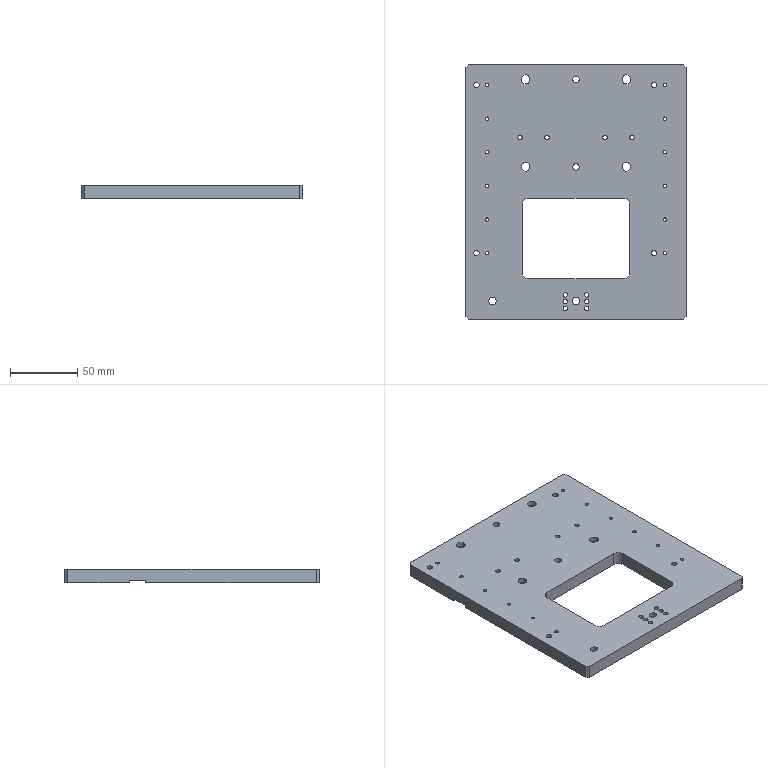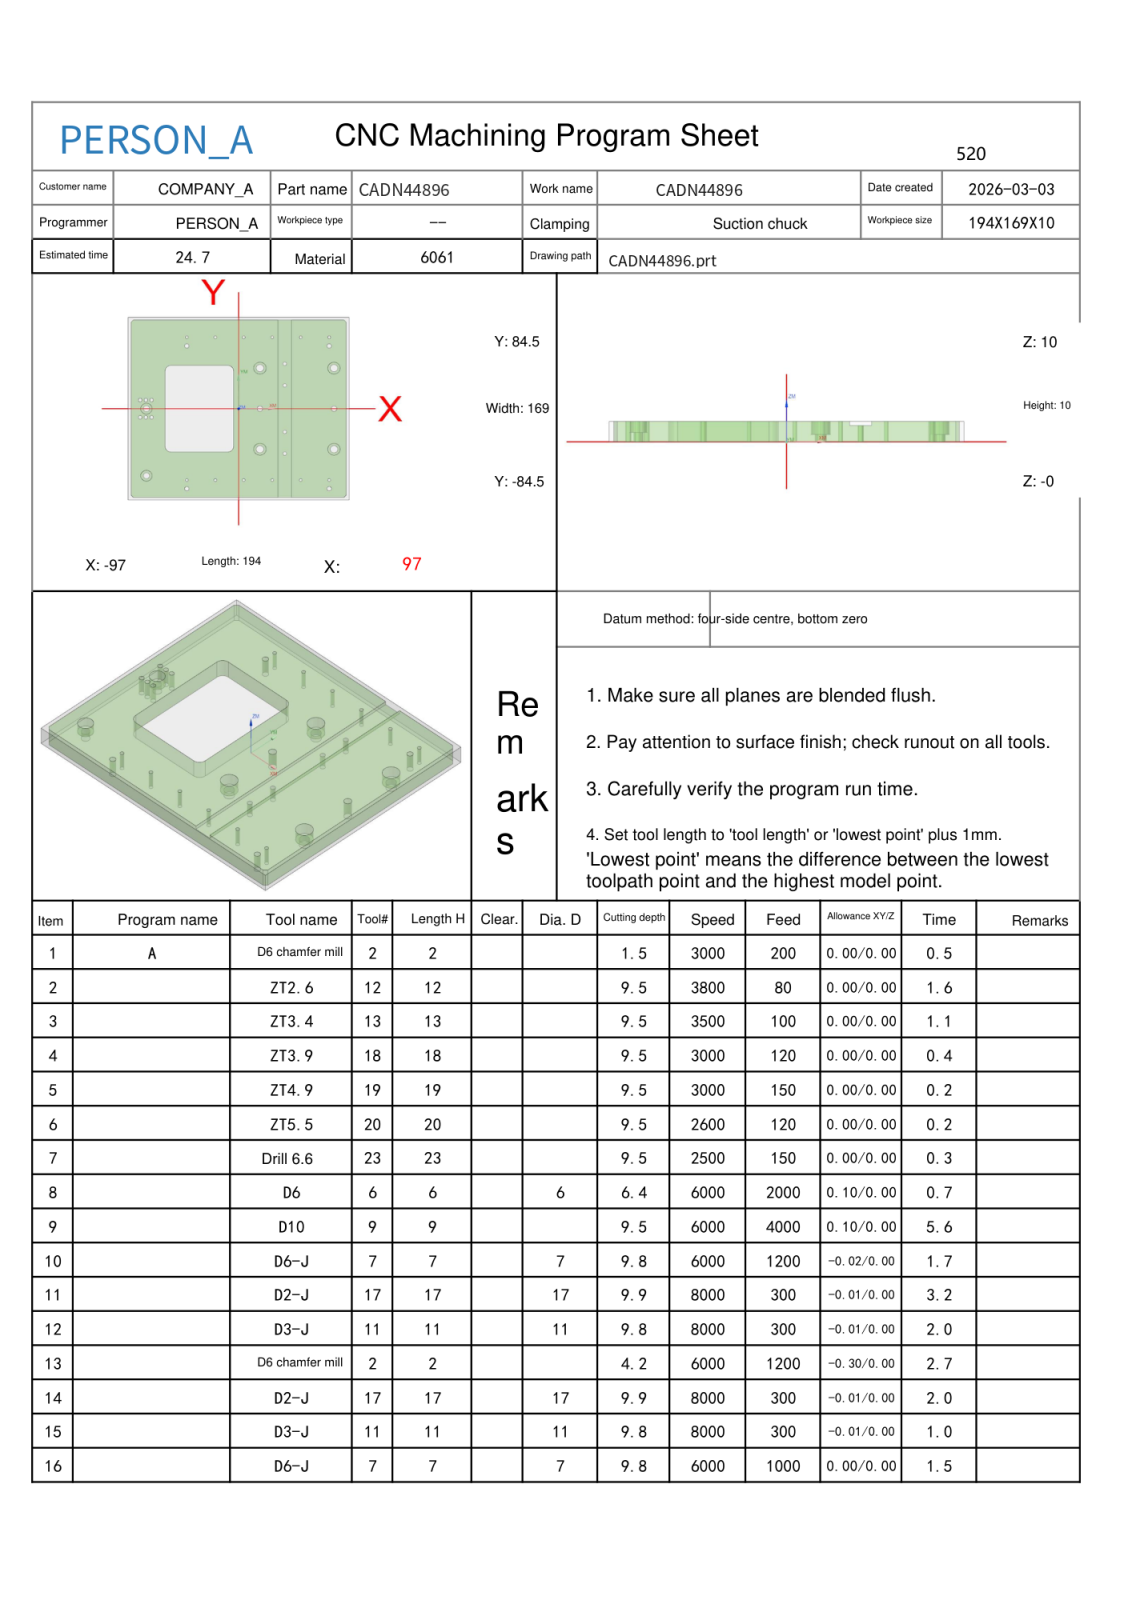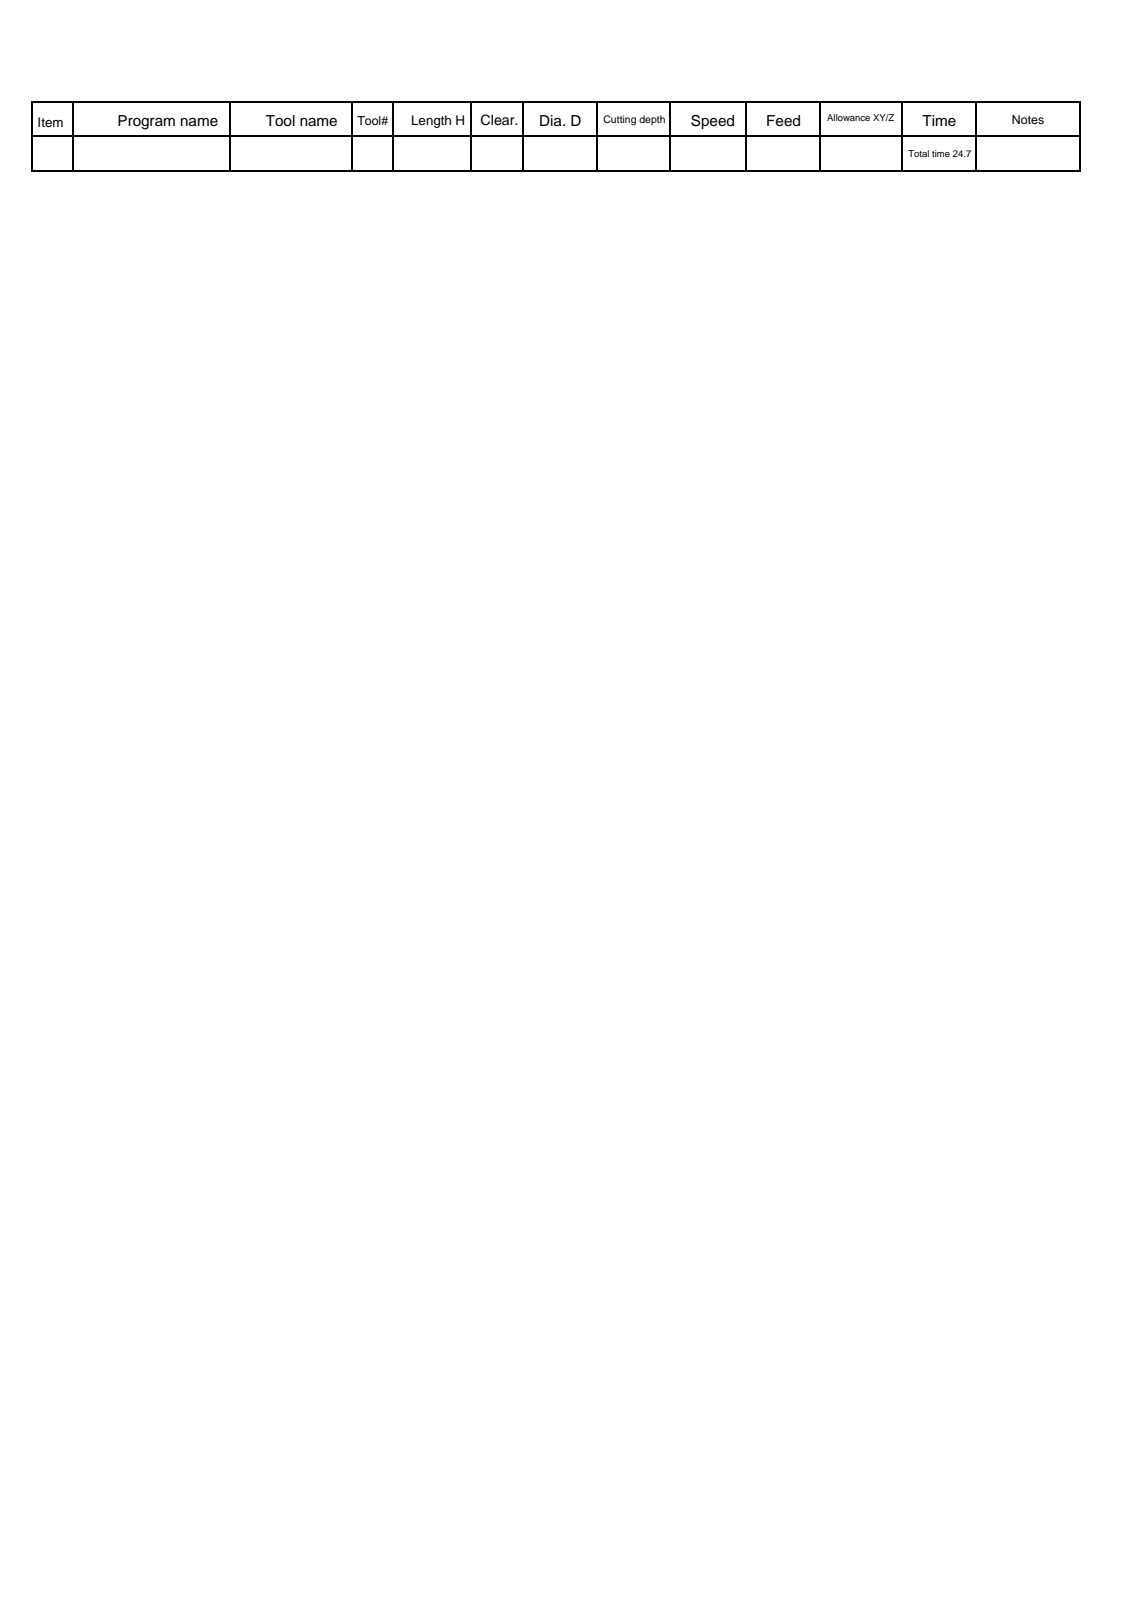NC program | NX | posted by the shop | part box 164 x 189 x 10 mm
Lines 1039 to 2443 of 4061, first 1137 of 1405 lines:
N11 T17 M06
(D2-J  D=2. R=0. H=17 ce=-0.01 di=0.00)
(D.N=17 MAX_Z=40. MIN_Z=0.15 Time=3.12M)
G00 G90 G54 X-75.935 Y8.28 M03 S8000
G43 H17 Z40.
M08
Z10.5
G01 X-76.054 Y8.446 Z10.489 F300.
X-76.222 Y8.566 Z10.478
X-76.421 Y8.626 Z10.468
X-76.579 Z10.459
X-76.77 Y8.57 Z10.449
X-76.933 Y8.458 Z10.439
X-77.054 Y8.301 Z10.428
X-77.12 Y8.114 Z10.418
X-77.126 Y7.921 Z10.408
X-77.066 Y7.722 Z10.397
X-76.946 Y7.554 Z10.386
X-76.778 Y7.434 Z10.375
X-76.579 Y7.374 Z10.364
X-76.421 Z10.356
X-76.222 Y7.434 Z10.345
X-76.054 Y7.554 Z10.334
X-75.934 Y7.722 Z10.323
X-75.874 Y7.921 Z10.313
Y8.079 Z10.304
X-75.934 Y8.278 Z10.293
X-76.054 Y8.446 Z10.282
X-76.222 Y8.566 Z10.272
X-76.421 Y8.626 Z10.261
X-76.579 Z10.252
X-76.77 Y8.57 Z10.242
X-76.933 Y8.458 Z10.232
X-77.054 Y8.301 Z10.221
X-77.12 Y8.114 Z10.211
X-77.126 Y7.921 Z10.201
X-77.066 Y7.722 Z10.19
X-76.946 Y7.554 Z10.179
X-76.778 Y7.434 Z10.168
X-76.579 Y7.374 Z10.157
X-76.421 Z10.149
X-76.222 Y7.434 Z10.138
X-76.054 Y7.554 Z10.127
X-75.934 Y7.722 Z10.117
X-75.874 Y7.921 Z10.106
Y8.079 Z10.097
X-75.934 Y8.278 Z10.087
X-76.054 Y8.446 Z10.076
X-76.222 Y8.566 Z10.065
X-76.421 Y8.626 Z10.054
X-76.579 Z10.046
X-76.77 Y8.57 Z10.035
X-76.933 Y8.458 Z10.025
X-77.054 Y8.301 Z10.015
X-77.12 Y8.114 Z10.004
X-77.125 Y8.035 Z10.
G41 D17
X-77.16 Y8.
G03 X-76.5 Y7.34 Z9.877 I.66 J0.0
X-75.84 Y8. Z9.754 I0.0 J.66
X-76.5 Y8.66 Z9.631 I-.66 J0.0
X-77.16 Y8. Z9.508 I0.0 J-.66
X-76.5 Y7.34 Z9.384 I.66 J0.0
X-75.84 Y8. Z9.261 I0.0 J.66
X-76.5 Y8.66 Z9.138 I-.66 J0.0
X-77.16 Y8. Z9.015 I0.0 J-.66
X-76.5 Y7.34 Z8.892 I.66 J0.0
X-75.84 Y8. Z8.769 I0.0 J.66
X-76.5 Y8.66 Z8.646 I-.66 J0.0
X-77.16 Y8. Z8.523 I0.0 J-.66
X-76.5 Y7.34 Z8.399 I.66 J0.0
X-75.84 Y8. Z8.276 I0.0 J.66
X-76.5 Y8.66 Z8.153 I-.66 J0.0
X-77.16 Y8. Z8.03 I0.0 J-.66
X-76.5 Y7.34 Z7.907 I.66 J0.0
X-75.84 Y8. Z7.784 I0.0 J.66
X-76.5 Y8.66 Z7.661 I-.66 J0.0
X-77.16 Y8. Z7.538 I0.0 J-.66
X-76.5 Y7.34 Z7.414 I.66 J0.0
X-75.84 Y8. Z7.291 I0.0 J.66
X-76.5 Y8.66 Z7.168 I-.66 J0.0
X-77.16 Y8. Z7.045 I0.0 J-.66
X-76.5 Y7.34 Z6.922 I.66 J0.0
X-75.84 Y8. Z6.799 I0.0 J.66
X-76.5 Y8.66 Z6.676 I-.66 J0.0
X-77.16 Y8. Z6.553 I0.0 J-.66
X-76.5 Y7.34 Z6.429 I.66 J0.0
X-75.84 Y8. Z6.306 I0.0 J.66
X-76.5 Y8.66 Z6.183 I-.66 J0.0
X-77.16 Y8. Z6.06 I0.0 J-.66
X-76.5 Y7.34 Z5.937 I.66 J0.0
X-75.84 Y8. Z5.814 I0.0 J.66
X-76.5 Y8.66 Z5.691 I-.66 J0.0
X-77.16 Y8. Z5.568 I0.0 J-.66
X-76.5 Y7.34 Z5.444 I.66 J0.0
X-75.84 Y8. Z5.321 I0.0 J.66
X-76.5 Y8.66 Z5.198 I-.66 J0.0
X-77.16 Y8. Z5.075 I0.0 J-.66
X-76.5 Y7.34 Z4.952 I.66 J0.0
X-75.84 Y8. Z4.829 I0.0 J.66
X-76.5 Y8.66 Z4.706 I-.66 J0.0
X-77.16 Y8. Z4.583 I0.0 J-.66
X-76.5 Y7.34 Z4.459 I.66 J0.0
X-75.84 Y8. Z4.336 I0.0 J.66
X-76.5 Y8.66 Z4.213 I-.66 J0.0
X-77.16 Y8. Z4.09 I0.0 J-.66
X-76.5 Y7.34 Z3.967 I.66 J0.0
X-75.84 Y8. Z3.844 I0.0 J.66
X-76.5 Y8.66 Z3.721 I-.66 J0.0
X-77.16 Y8. Z3.598 I0.0 J-.66
X-76.5 Y7.34 Z3.474 I.66 J0.0
X-75.84 Y8. Z3.351 I0.0 J.66
X-76.5 Y8.66 Z3.228 I-.66 J0.0
X-77.16 Y8. Z3.105 I0.0 J-.66
X-76.5 Y7.34 Z2.982 I.66 J0.0
X-75.84 Y8. Z2.859 I0.0 J.66
X-76.5 Y8.66 Z2.736 I-.66 J0.0
X-77.16 Y8. Z2.613 I0.0 J-.66
X-76.5 Y7.34 Z2.489 I.66 J0.0
X-75.84 Y8. Z2.366 I0.0 J.66
X-76.5 Y8.66 Z2.243 I-.66 J0.0
X-77.16 Y8. Z2.12 I0.0 J-.66
X-76.5 Y7.34 Z1.997 I.66 J0.0
X-75.84 Y8. Z1.874 I0.0 J.66
X-76.5 Y8.66 Z1.751 I-.66 J0.0
X-77.16 Y8. Z1.628 I0.0 J-.66
X-76.5 Y7.34 Z1.504 I.66 J0.0
X-75.84 Y8. Z1.381 I0.0 J.66
X-76.5 Y8.66 Z1.258 I-.66 J0.0
X-77.16 Y8. Z1.135 I0.0 J-.66
X-76.5 Y7.34 Z1.012 I.66 J0.0
X-75.84 Y8. Z.889 I0.0 J.66
X-76.5 Y8.66 Z.766 I-.66 J0.0
X-77.16 Y8. Z.643 I0.0 J-.66
X-76.5 Y7.34 Z.519 I.66 J0.0
X-75.84 Y8. Z.396 I0.0 J.66
X-76.5 Y8.66 Z.273 I-.66 J0.0
X-77.16 Y8. Z.15 I0.0 J-.66
X-76.5 Y7.34 I.66 J0.0
X-75.84 Y8. I0.0 J.66
X-76.5 Y8.66 I-.66 J0.0
X-77.16 Y8. I0.0 J-.66
X-77.042 Y7.624 I.66 J0.0
G01 X-77.025 Y7.603
X-76.997 Y7.598
X-76.973 Y7.611
G40 X-76.932 Y7.64
Z1.15
G00 Z40.
X-80.935 Y8.28
Z10.5
G01 X-81.054 Y8.446 Z10.489
X-81.222 Y8.566 Z10.478
X-81.421 Y8.626 Z10.468
X-81.579 Z10.459
X-81.77 Y8.57 Z10.449
X-81.933 Y8.458 Z10.439
X-82.054 Y8.301 Z10.428
X-82.12 Y8.114 Z10.418
X-82.126 Y7.921 Z10.408
X-82.066 Y7.722 Z10.397
X-81.946 Y7.554 Z10.386
X-81.778 Y7.434 Z10.375
X-81.579 Y7.374 Z10.364
X-81.421 Z10.356
X-81.222 Y7.434 Z10.345
X-81.054 Y7.554 Z10.334
X-80.934 Y7.722 Z10.323
X-80.874 Y7.921 Z10.313
Y8.079 Z10.304
X-80.934 Y8.278 Z10.293
X-81.054 Y8.446 Z10.282
X-81.222 Y8.566 Z10.272
X-81.421 Y8.626 Z10.261
X-81.579 Z10.252
X-81.77 Y8.57 Z10.242
X-81.933 Y8.458 Z10.232
X-82.054 Y8.301 Z10.221
X-82.12 Y8.114 Z10.211
X-82.126 Y7.921 Z10.201
X-82.066 Y7.722 Z10.19
X-81.946 Y7.554 Z10.179
X-81.778 Y7.434 Z10.168
X-81.579 Y7.374 Z10.157
X-81.421 Z10.149
X-81.222 Y7.434 Z10.138
X-81.054 Y7.554 Z10.127
X-80.934 Y7.722 Z10.117
X-80.874 Y7.921 Z10.106
Y8.079 Z10.097
X-80.934 Y8.278 Z10.087
X-81.054 Y8.446 Z10.076
X-81.222 Y8.566 Z10.065
X-81.421 Y8.626 Z10.054
X-81.579 Z10.046
X-81.77 Y8.57 Z10.035
X-81.933 Y8.458 Z10.025
X-82.054 Y8.301 Z10.015
X-82.12 Y8.114 Z10.004
X-82.125 Y8.035 Z10.
G41 D17
X-82.16 Y8.
G03 X-81.5 Y7.34 Z9.877 I.66 J0.0
X-80.84 Y8. Z9.754 I0.0 J.66
X-81.5 Y8.66 Z9.631 I-.66 J0.0
X-82.16 Y8. Z9.508 I0.0 J-.66
X-81.5 Y7.34 Z9.384 I.66 J0.0
X-80.84 Y8. Z9.261 I0.0 J.66
X-81.5 Y8.66 Z9.138 I-.66 J0.0
X-82.16 Y8. Z9.015 I0.0 J-.66
X-81.5 Y7.34 Z8.892 I.66 J0.0
X-80.84 Y8. Z8.769 I0.0 J.66
X-81.5 Y8.66 Z8.646 I-.66 J0.0
X-82.16 Y8. Z8.523 I0.0 J-.66
X-81.5 Y7.34 Z8.399 I.66 J0.0
X-80.84 Y8. Z8.276 I0.0 J.66
X-81.5 Y8.66 Z8.153 I-.66 J0.0
X-82.16 Y8. Z8.03 I0.0 J-.66
X-81.5 Y7.34 Z7.907 I.66 J0.0
X-80.84 Y8. Z7.784 I0.0 J.66
X-81.5 Y8.66 Z7.661 I-.66 J0.0
X-82.16 Y8. Z7.538 I0.0 J-.66
X-81.5 Y7.34 Z7.414 I.66 J0.0
X-80.84 Y8. Z7.291 I0.0 J.66
X-81.5 Y8.66 Z7.168 I-.66 J0.0
X-82.16 Y8. Z7.045 I0.0 J-.66
X-81.5 Y7.34 Z6.922 I.66 J0.0
X-80.84 Y8. Z6.799 I0.0 J.66
X-81.5 Y8.66 Z6.676 I-.66 J0.0
X-82.16 Y8. Z6.553 I0.0 J-.66
X-81.5 Y7.34 Z6.429 I.66 J0.0
X-80.84 Y8. Z6.306 I0.0 J.66
X-81.5 Y8.66 Z6.183 I-.66 J0.0
X-82.16 Y8. Z6.06 I0.0 J-.66
X-81.5 Y7.34 Z5.937 I.66 J0.0
X-80.84 Y8. Z5.814 I0.0 J.66
X-81.5 Y8.66 Z5.691 I-.66 J0.0
X-82.16 Y8. Z5.568 I0.0 J-.66
X-81.5 Y7.34 Z5.444 I.66 J0.0
X-80.84 Y8. Z5.321 I0.0 J.66
X-81.5 Y8.66 Z5.198 I-.66 J0.0
X-82.16 Y8. Z5.075 I0.0 J-.66
X-81.5 Y7.34 Z4.952 I.66 J0.0
X-80.84 Y8. Z4.829 I0.0 J.66
X-81.5 Y8.66 Z4.706 I-.66 J0.0
X-82.16 Y8. Z4.583 I0.0 J-.66
X-81.5 Y7.34 Z4.459 I.66 J0.0
X-80.84 Y8. Z4.336 I0.0 J.66
X-81.5 Y8.66 Z4.213 I-.66 J0.0
X-82.16 Y8. Z4.09 I0.0 J-.66
X-81.5 Y7.34 Z3.967 I.66 J0.0
X-80.84 Y8. Z3.844 I0.0 J.66
X-81.5 Y8.66 Z3.721 I-.66 J0.0
X-82.16 Y8. Z3.598 I0.0 J-.66
X-81.5 Y7.34 Z3.474 I.66 J0.0
X-80.84 Y8. Z3.351 I0.0 J.66
X-81.5 Y8.66 Z3.228 I-.66 J0.0
X-82.16 Y8. Z3.105 I0.0 J-.66
X-81.5 Y7.34 Z2.982 I.66 J0.0
X-80.84 Y8. Z2.859 I0.0 J.66
X-81.5 Y8.66 Z2.736 I-.66 J0.0
X-82.16 Y8. Z2.613 I0.0 J-.66
X-81.5 Y7.34 Z2.489 I.66 J0.0
X-80.84 Y8. Z2.366 I0.0 J.66
X-81.5 Y8.66 Z2.243 I-.66 J0.0
X-82.16 Y8. Z2.12 I0.0 J-.66
X-81.5 Y7.34 Z1.997 I.66 J0.0
X-80.84 Y8. Z1.874 I0.0 J.66
X-81.5 Y8.66 Z1.751 I-.66 J0.0
X-82.16 Y8. Z1.628 I0.0 J-.66
X-81.5 Y7.34 Z1.504 I.66 J0.0
X-80.84 Y8. Z1.381 I0.0 J.66
X-81.5 Y8.66 Z1.258 I-.66 J0.0
X-82.16 Y8. Z1.135 I0.0 J-.66
X-81.5 Y7.34 Z1.012 I.66 J0.0
X-80.84 Y8. Z.889 I0.0 J.66
X-81.5 Y8.66 Z.766 I-.66 J0.0
X-82.16 Y8. Z.643 I0.0 J-.66
X-81.5 Y7.34 Z.519 I.66 J0.0
X-80.84 Y8. Z.396 I0.0 J.66
X-81.5 Y8.66 Z.273 I-.66 J0.0
X-82.16 Y8. Z.15 I0.0 J-.66
X-81.5 Y7.34 I.66 J0.0
X-80.84 Y8. I0.0 J.66
X-81.5 Y8.66 I-.66 J0.0
X-82.16 Y8. I0.0 J-.66
X-82.042 Y7.624 I.66 J0.0
G01 X-82.025 Y7.603
X-81.997 Y7.598
X-81.973 Y7.611
G40 X-81.932 Y7.64
Z1.15
G00 Z40.
X-85.935 Y8.28
Z10.5
G01 X-86.054 Y8.446 Z10.489
X-86.222 Y8.566 Z10.478
X-86.421 Y8.626 Z10.468
X-86.579 Z10.459
X-86.77 Y8.57 Z10.449
X-86.933 Y8.458 Z10.439
X-87.054 Y8.301 Z10.428
X-87.12 Y8.114 Z10.418
X-87.126 Y7.921 Z10.408
X-87.066 Y7.722 Z10.397
X-86.946 Y7.554 Z10.386
X-86.778 Y7.434 Z10.375
X-86.579 Y7.374 Z10.364
X-86.421 Z10.356
X-86.222 Y7.434 Z10.345
X-86.054 Y7.554 Z10.334
X-85.934 Y7.722 Z10.323
X-85.874 Y7.921 Z10.313
Y8.079 Z10.304
X-85.934 Y8.278 Z10.293
X-86.054 Y8.446 Z10.282
X-86.222 Y8.566 Z10.272
X-86.421 Y8.626 Z10.261
X-86.579 Z10.252
X-86.77 Y8.57 Z10.242
X-86.933 Y8.458 Z10.232
X-87.054 Y8.301 Z10.221
X-87.12 Y8.114 Z10.211
X-87.126 Y7.921 Z10.201
X-87.066 Y7.722 Z10.19
X-86.946 Y7.554 Z10.179
X-86.778 Y7.434 Z10.168
X-86.579 Y7.374 Z10.157
X-86.421 Z10.149
X-86.222 Y7.434 Z10.138
X-86.054 Y7.554 Z10.127
X-85.934 Y7.722 Z10.117
X-85.874 Y7.921 Z10.106
Y8.079 Z10.097
X-85.934 Y8.278 Z10.087
X-86.054 Y8.446 Z10.076
X-86.222 Y8.566 Z10.065
X-86.421 Y8.626 Z10.054
X-86.579 Z10.046
X-86.77 Y8.57 Z10.035
X-86.933 Y8.458 Z10.025
X-87.054 Y8.301 Z10.015
X-87.12 Y8.114 Z10.004
X-87.125 Y8.035 Z10.
G41 D17
X-87.16 Y8.
G03 X-86.5 Y7.34 Z9.877 I.66 J0.0
X-85.84 Y8. Z9.754 I0.0 J.66
X-86.5 Y8.66 Z9.631 I-.66 J0.0
X-87.16 Y8. Z9.508 I0.0 J-.66
X-86.5 Y7.34 Z9.384 I.66 J0.0
X-85.84 Y8. Z9.261 I0.0 J.66
X-86.5 Y8.66 Z9.138 I-.66 J0.0
X-87.16 Y8. Z9.015 I0.0 J-.66
X-86.5 Y7.34 Z8.892 I.66 J0.0
X-85.84 Y8. Z8.769 I0.0 J.66
X-86.5 Y8.66 Z8.646 I-.66 J0.0
X-87.16 Y8. Z8.523 I0.0 J-.66
X-86.5 Y7.34 Z8.399 I.66 J0.0
X-85.84 Y8. Z8.276 I0.0 J.66
X-86.5 Y8.66 Z8.153 I-.66 J0.0
X-87.16 Y8. Z8.03 I0.0 J-.66
X-86.5 Y7.34 Z7.907 I.66 J0.0
X-85.84 Y8. Z7.784 I0.0 J.66
X-86.5 Y8.66 Z7.661 I-.66 J0.0
X-87.16 Y8. Z7.538 I0.0 J-.66
X-86.5 Y7.34 Z7.414 I.66 J0.0
X-85.84 Y8. Z7.291 I0.0 J.66
X-86.5 Y8.66 Z7.168 I-.66 J0.0
X-87.16 Y8. Z7.045 I0.0 J-.66
X-86.5 Y7.34 Z6.922 I.66 J0.0
X-85.84 Y8. Z6.799 I0.0 J.66
X-86.5 Y8.66 Z6.676 I-.66 J0.0
X-87.16 Y8. Z6.553 I0.0 J-.66
X-86.5 Y7.34 Z6.429 I.66 J0.0
X-85.84 Y8. Z6.306 I0.0 J.66
X-86.5 Y8.66 Z6.183 I-.66 J0.0
X-87.16 Y8. Z6.06 I0.0 J-.66
X-86.5 Y7.34 Z5.937 I.66 J0.0
X-85.84 Y8. Z5.814 I0.0 J.66
X-86.5 Y8.66 Z5.691 I-.66 J0.0
X-87.16 Y8. Z5.568 I0.0 J-.66
X-86.5 Y7.34 Z5.444 I.66 J0.0
X-85.84 Y8. Z5.321 I0.0 J.66
X-86.5 Y8.66 Z5.198 I-.66 J0.0
X-87.16 Y8. Z5.075 I0.0 J-.66
X-86.5 Y7.34 Z4.952 I.66 J0.0
X-85.84 Y8. Z4.829 I0.0 J.66
X-86.5 Y8.66 Z4.706 I-.66 J0.0
X-87.16 Y8. Z4.583 I0.0 J-.66
X-86.5 Y7.34 Z4.459 I.66 J0.0
X-85.84 Y8. Z4.336 I0.0 J.66
X-86.5 Y8.66 Z4.213 I-.66 J0.0
X-87.16 Y8. Z4.09 I0.0 J-.66
X-86.5 Y7.34 Z3.967 I.66 J0.0
X-85.84 Y8. Z3.844 I0.0 J.66
X-86.5 Y8.66 Z3.721 I-.66 J0.0
X-87.16 Y8. Z3.598 I0.0 J-.66
X-86.5 Y7.34 Z3.474 I.66 J0.0
X-85.84 Y8. Z3.351 I0.0 J.66
X-86.5 Y8.66 Z3.228 I-.66 J0.0
X-87.16 Y8. Z3.105 I0.0 J-.66
X-86.5 Y7.34 Z2.982 I.66 J0.0
X-85.84 Y8. Z2.859 I0.0 J.66
X-86.5 Y8.66 Z2.736 I-.66 J0.0
X-87.16 Y8. Z2.613 I0.0 J-.66
X-86.5 Y7.34 Z2.489 I.66 J0.0
X-85.84 Y8. Z2.366 I0.0 J.66
X-86.5 Y8.66 Z2.243 I-.66 J0.0
X-87.16 Y8. Z2.12 I0.0 J-.66
X-86.5 Y7.34 Z1.997 I.66 J0.0
X-85.84 Y8. Z1.874 I0.0 J.66
X-86.5 Y8.66 Z1.751 I-.66 J0.0
X-87.16 Y8. Z1.628 I0.0 J-.66
X-86.5 Y7.34 Z1.504 I.66 J0.0
X-85.84 Y8. Z1.381 I0.0 J.66
X-86.5 Y8.66 Z1.258 I-.66 J0.0
X-87.16 Y8. Z1.135 I0.0 J-.66
X-86.5 Y7.34 Z1.012 I.66 J0.0
X-85.84 Y8. Z.889 I0.0 J.66
X-86.5 Y8.66 Z.766 I-.66 J0.0
X-87.16 Y8. Z.643 I0.0 J-.66
X-86.5 Y7.34 Z.519 I.66 J0.0
X-85.84 Y8. Z.396 I0.0 J.66
X-86.5 Y8.66 Z.273 I-.66 J0.0
X-87.16 Y8. Z.15 I0.0 J-.66
X-86.5 Y7.34 I.66 J0.0
X-85.84 Y8. I0.0 J.66
X-86.5 Y8.66 I-.66 J0.0
X-87.16 Y8. I0.0 J-.66
X-87.042 Y7.624 I.66 J0.0
G01 X-87.025 Y7.603
X-86.997 Y7.598
X-86.973 Y7.611
G40 X-86.932 Y7.64
Z1.15
G00 Z40.
X-85.935 Y-7.72
Z10.5
G01 X-86.054 Y-7.554 Z10.489
X-86.222 Y-7.434 Z10.478
X-86.421 Y-7.374 Z10.468
X-86.579 Z10.459
X-86.77 Y-7.43 Z10.449
X-86.933 Y-7.542 Z10.439
X-87.054 Y-7.699 Z10.428
X-87.12 Y-7.886 Z10.418
X-87.126 Y-8.079 Z10.408
X-87.066 Y-8.278 Z10.397
X-86.946 Y-8.446 Z10.386
X-86.778 Y-8.566 Z10.375
X-86.579 Y-8.626 Z10.364
X-86.421 Z10.356
X-86.222 Y-8.566 Z10.345
X-86.054 Y-8.446 Z10.334
X-85.934 Y-8.278 Z10.323
X-85.874 Y-8.079 Z10.313
Y-7.921 Z10.304
X-85.934 Y-7.722 Z10.293
X-86.054 Y-7.554 Z10.282
X-86.222 Y-7.434 Z10.272
X-86.421 Y-7.374 Z10.261
X-86.579 Z10.252
X-86.77 Y-7.43 Z10.242
X-86.933 Y-7.542 Z10.232
X-87.054 Y-7.699 Z10.221
X-87.12 Y-7.886 Z10.211
X-87.126 Y-8.079 Z10.201
X-87.066 Y-8.278 Z10.19
X-86.946 Y-8.446 Z10.179
X-86.778 Y-8.566 Z10.168
X-86.579 Y-8.626 Z10.157
X-86.421 Z10.149
X-86.222 Y-8.566 Z10.138
X-86.054 Y-8.446 Z10.127
X-85.934 Y-8.278 Z10.117
X-85.874 Y-8.079 Z10.106
Y-7.921 Z10.097
X-85.934 Y-7.722 Z10.087
X-86.054 Y-7.554 Z10.076
X-86.222 Y-7.434 Z10.065
X-86.421 Y-7.374 Z10.054
X-86.579 Z10.046
X-86.77 Y-7.43 Z10.035
X-86.933 Y-7.542 Z10.025
X-87.054 Y-7.699 Z10.015
X-87.12 Y-7.886 Z10.004
X-87.125 Y-7.965 Z10.
G41 D17
X-87.16 Y-8.
G03 X-86.5 Y-8.66 Z9.877 I.66 J0.0
X-85.84 Y-8. Z9.754 I0.0 J.66
X-86.5 Y-7.34 Z9.631 I-.66 J0.0
X-87.16 Y-8. Z9.508 I0.0 J-.66
X-86.5 Y-8.66 Z9.384 I.66 J0.0
X-85.84 Y-8. Z9.261 I0.0 J.66
X-86.5 Y-7.34 Z9.138 I-.66 J0.0
X-87.16 Y-8. Z9.015 I0.0 J-.66
X-86.5 Y-8.66 Z8.892 I.66 J0.0
X-85.84 Y-8. Z8.769 I0.0 J.66
X-86.5 Y-7.34 Z8.646 I-.66 J0.0
X-87.16 Y-8. Z8.523 I0.0 J-.66
X-86.5 Y-8.66 Z8.399 I.66 J0.0
X-85.84 Y-8. Z8.276 I0.0 J.66
X-86.5 Y-7.34 Z8.153 I-.66 J0.0
X-87.16 Y-8. Z8.03 I0.0 J-.66
X-86.5 Y-8.66 Z7.907 I.66 J0.0
X-85.84 Y-8. Z7.784 I0.0 J.66
X-86.5 Y-7.34 Z7.661 I-.66 J0.0
X-87.16 Y-8. Z7.538 I0.0 J-.66
X-86.5 Y-8.66 Z7.414 I.66 J0.0
X-85.84 Y-8. Z7.291 I0.0 J.66
X-86.5 Y-7.34 Z7.168 I-.66 J0.0
X-87.16 Y-8. Z7.045 I0.0 J-.66
X-86.5 Y-8.66 Z6.922 I.66 J0.0
X-85.84 Y-8. Z6.799 I0.0 J.66
X-86.5 Y-7.34 Z6.676 I-.66 J0.0
X-87.16 Y-8. Z6.553 I0.0 J-.66
X-86.5 Y-8.66 Z6.429 I.66 J0.0
X-85.84 Y-8. Z6.306 I0.0 J.66
X-86.5 Y-7.34 Z6.183 I-.66 J0.0
X-87.16 Y-8. Z6.06 I0.0 J-.66
X-86.5 Y-8.66 Z5.937 I.66 J0.0
X-85.84 Y-8. Z5.814 I0.0 J.66
X-86.5 Y-7.34 Z5.691 I-.66 J0.0
X-87.16 Y-8. Z5.568 I0.0 J-.66
X-86.5 Y-8.66 Z5.444 I.66 J0.0
X-85.84 Y-8. Z5.321 I0.0 J.66
X-86.5 Y-7.34 Z5.198 I-.66 J0.0
X-87.16 Y-8. Z5.075 I0.0 J-.66
X-86.5 Y-8.66 Z4.952 I.66 J0.0
X-85.84 Y-8. Z4.829 I0.0 J.66
X-86.5 Y-7.34 Z4.706 I-.66 J0.0
X-87.16 Y-8. Z4.583 I0.0 J-.66
X-86.5 Y-8.66 Z4.459 I.66 J0.0
X-85.84 Y-8. Z4.336 I0.0 J.66
X-86.5 Y-7.34 Z4.213 I-.66 J0.0
X-87.16 Y-8. Z4.09 I0.0 J-.66
X-86.5 Y-8.66 Z3.967 I.66 J0.0
X-85.84 Y-8. Z3.844 I0.0 J.66
X-86.5 Y-7.34 Z3.721 I-.66 J0.0
X-87.16 Y-8. Z3.598 I0.0 J-.66
X-86.5 Y-8.66 Z3.474 I.66 J0.0
X-85.84 Y-8. Z3.351 I0.0 J.66
X-86.5 Y-7.34 Z3.228 I-.66 J0.0
X-87.16 Y-8. Z3.105 I0.0 J-.66
X-86.5 Y-8.66 Z2.982 I.66 J0.0
X-85.84 Y-8. Z2.859 I0.0 J.66
X-86.5 Y-7.34 Z2.736 I-.66 J0.0
X-87.16 Y-8. Z2.613 I0.0 J-.66
X-86.5 Y-8.66 Z2.489 I.66 J0.0
X-85.84 Y-8. Z2.366 I0.0 J.66
X-86.5 Y-7.34 Z2.243 I-.66 J0.0
X-87.16 Y-8. Z2.12 I0.0 J-.66
X-86.5 Y-8.66 Z1.997 I.66 J0.0
X-85.84 Y-8. Z1.874 I0.0 J.66
X-86.5 Y-7.34 Z1.751 I-.66 J0.0
X-87.16 Y-8. Z1.628 I0.0 J-.66
X-86.5 Y-8.66 Z1.504 I.66 J0.0
X-85.84 Y-8. Z1.381 I0.0 J.66
X-86.5 Y-7.34 Z1.258 I-.66 J0.0
X-87.16 Y-8. Z1.135 I0.0 J-.66
X-86.5 Y-8.66 Z1.012 I.66 J0.0
X-85.84 Y-8. Z.889 I0.0 J.66
X-86.5 Y-7.34 Z.766 I-.66 J0.0
X-87.16 Y-8. Z.643 I0.0 J-.66
X-86.5 Y-8.66 Z.519 I.66 J0.0
X-85.84 Y-8. Z.396 I0.0 J.66
X-86.5 Y-7.34 Z.273 I-.66 J0.0
X-87.16 Y-8. Z.15 I0.0 J-.66
X-86.5 Y-8.66 I.66 J0.0
X-85.84 Y-8. I0.0 J.66
X-86.5 Y-7.34 I-.66 J0.0
X-87.16 Y-8. I0.0 J-.66
X-87.042 Y-8.376 I.66 J0.0
G01 X-87.025 Y-8.397
X-86.997 Y-8.402
X-86.973 Y-8.389
G40 X-86.932 Y-8.36
Z1.15
G00 Z40.
X-80.935 Y-7.72
Z10.5
G01 X-81.054 Y-7.554 Z10.489
X-81.222 Y-7.434 Z10.478
X-81.421 Y-7.374 Z10.468
X-81.579 Z10.459
X-81.77 Y-7.43 Z10.449
X-81.933 Y-7.542 Z10.439
X-82.054 Y-7.699 Z10.428
X-82.12 Y-7.886 Z10.418
X-82.126 Y-8.079 Z10.408
X-82.066 Y-8.278 Z10.397
X-81.946 Y-8.446 Z10.386
X-81.778 Y-8.566 Z10.375
X-81.579 Y-8.626 Z10.364
X-81.421 Z10.356
X-81.222 Y-8.566 Z10.345
X-81.054 Y-8.446 Z10.334
X-80.934 Y-8.278 Z10.323
X-80.874 Y-8.079 Z10.313
Y-7.921 Z10.304
X-80.934 Y-7.722 Z10.293
X-81.054 Y-7.554 Z10.282
X-81.222 Y-7.434 Z10.272
X-81.421 Y-7.374 Z10.261
X-81.579 Z10.252
X-81.77 Y-7.43 Z10.242
X-81.933 Y-7.542 Z10.232
X-82.054 Y-7.699 Z10.221
X-82.12 Y-7.886 Z10.211
X-82.126 Y-8.079 Z10.201
X-82.066 Y-8.278 Z10.19
X-81.946 Y-8.446 Z10.179
X-81.778 Y-8.566 Z10.168
X-81.579 Y-8.626 Z10.157
X-81.421 Z10.149
X-81.222 Y-8.566 Z10.138
X-81.054 Y-8.446 Z10.127
X-80.934 Y-8.278 Z10.117
X-80.874 Y-8.079 Z10.106
Y-7.921 Z10.097
X-80.934 Y-7.722 Z10.087
X-81.054 Y-7.554 Z10.076
X-81.222 Y-7.434 Z10.065
X-81.421 Y-7.374 Z10.054
X-81.579 Z10.046
X-81.77 Y-7.43 Z10.035
X-81.933 Y-7.542 Z10.025
X-82.054 Y-7.699 Z10.015
X-82.12 Y-7.886 Z10.004
X-82.125 Y-7.965 Z10.
G41 D17
X-82.16 Y-8.
G03 X-81.5 Y-8.66 Z9.877 I.66 J0.0
X-80.84 Y-8. Z9.754 I0.0 J.66
X-81.5 Y-7.34 Z9.631 I-.66 J0.0
X-82.16 Y-8. Z9.508 I0.0 J-.66
X-81.5 Y-8.66 Z9.384 I.66 J0.0
X-80.84 Y-8. Z9.261 I0.0 J.66
X-81.5 Y-7.34 Z9.138 I-.66 J0.0
X-82.16 Y-8. Z9.015 I0.0 J-.66
X-81.5 Y-8.66 Z8.892 I.66 J0.0
X-80.84 Y-8. Z8.769 I0.0 J.66
X-81.5 Y-7.34 Z8.646 I-.66 J0.0
X-82.16 Y-8. Z8.523 I0.0 J-.66
X-81.5 Y-8.66 Z8.399 I.66 J0.0
X-80.84 Y-8. Z8.276 I0.0 J.66
X-81.5 Y-7.34 Z8.153 I-.66 J0.0
X-82.16 Y-8. Z8.03 I0.0 J-.66
X-81.5 Y-8.66 Z7.907 I.66 J0.0
X-80.84 Y-8. Z7.784 I0.0 J.66
X-81.5 Y-7.34 Z7.661 I-.66 J0.0
X-82.16 Y-8. Z7.538 I0.0 J-.66
X-81.5 Y-8.66 Z7.414 I.66 J0.0
X-80.84 Y-8. Z7.291 I0.0 J.66
X-81.5 Y-7.34 Z7.168 I-.66 J0.0
X-82.16 Y-8. Z7.045 I0.0 J-.66
X-81.5 Y-8.66 Z6.922 I.66 J0.0
X-80.84 Y-8. Z6.799 I0.0 J.66
X-81.5 Y-7.34 Z6.676 I-.66 J0.0
X-82.16 Y-8. Z6.553 I0.0 J-.66
X-81.5 Y-8.66 Z6.429 I.66 J0.0
X-80.84 Y-8. Z6.306 I0.0 J.66
X-81.5 Y-7.34 Z6.183 I-.66 J0.0
X-82.16 Y-8. Z6.06 I0.0 J-.66
X-81.5 Y-8.66 Z5.937 I.66 J0.0
X-80.84 Y-8. Z5.814 I0.0 J.66
X-81.5 Y-7.34 Z5.691 I-.66 J0.0
X-82.16 Y-8. Z5.568 I0.0 J-.66
X-81.5 Y-8.66 Z5.444 I.66 J0.0
X-80.84 Y-8. Z5.321 I0.0 J.66
X-81.5 Y-7.34 Z5.198 I-.66 J0.0
X-82.16 Y-8. Z5.075 I0.0 J-.66
X-81.5 Y-8.66 Z4.952 I.66 J0.0
X-80.84 Y-8. Z4.829 I0.0 J.66
X-81.5 Y-7.34 Z4.706 I-.66 J0.0
X-82.16 Y-8. Z4.583 I0.0 J-.66
X-81.5 Y-8.66 Z4.459 I.66 J0.0
X-80.84 Y-8. Z4.336 I0.0 J.66
X-81.5 Y-7.34 Z4.213 I-.66 J0.0
X-82.16 Y-8. Z4.09 I0.0 J-.66
X-81.5 Y-8.66 Z3.967 I.66 J0.0
X-80.84 Y-8. Z3.844 I0.0 J.66
X-81.5 Y-7.34 Z3.721 I-.66 J0.0
X-82.16 Y-8. Z3.598 I0.0 J-.66
X-81.5 Y-8.66 Z3.474 I.66 J0.0
X-80.84 Y-8. Z3.351 I0.0 J.66
X-81.5 Y-7.34 Z3.228 I-.66 J0.0
X-82.16 Y-8. Z3.105 I0.0 J-.66
X-81.5 Y-8.66 Z2.982 I.66 J0.0
X-80.84 Y-8. Z2.859 I0.0 J.66
X-81.5 Y-7.34 Z2.736 I-.66 J0.0
X-82.16 Y-8. Z2.613 I0.0 J-.66
X-81.5 Y-8.66 Z2.489 I.66 J0.0
X-80.84 Y-8. Z2.366 I0.0 J.66
X-81.5 Y-7.34 Z2.243 I-.66 J0.0
X-82.16 Y-8. Z2.12 I0.0 J-.66
X-81.5 Y-8.66 Z1.997 I.66 J0.0
X-80.84 Y-8. Z1.874 I0.0 J.66
X-81.5 Y-7.34 Z1.751 I-.66 J0.0
X-82.16 Y-8. Z1.628 I0.0 J-.66
X-81.5 Y-8.66 Z1.504 I.66 J0.0
X-80.84 Y-8. Z1.381 I0.0 J.66
X-81.5 Y-7.34 Z1.258 I-.66 J0.0
X-82.16 Y-8. Z1.135 I0.0 J-.66
X-81.5 Y-8.66 Z1.012 I.66 J0.0
X-80.84 Y-8. Z.889 I0.0 J.66
X-81.5 Y-7.34 Z.766 I-.66 J0.0
X-82.16 Y-8. Z.643 I0.0 J-.66
X-81.5 Y-8.66 Z.519 I.66 J0.0
X-80.84 Y-8. Z.396 I0.0 J.66
X-81.5 Y-7.34 Z.273 I-.66 J0.0
X-82.16 Y-8. Z.15 I0.0 J-.66
X-81.5 Y-8.66 I.66 J0.0
X-80.84 Y-8. I0.0 J.66
X-81.5 Y-7.34 I-.66 J0.0
X-82.16 Y-8. I0.0 J-.66
X-82.042 Y-8.376 I.66 J0.0
G01 X-82.025 Y-8.397
X-81.997 Y-8.402
X-81.973 Y-8.389
G40 X-81.932 Y-8.36
Z1.15
G00 Z40.
X-75.935 Y-7.72
Z10.5
G01 X-76.054 Y-7.554 Z10.489
X-76.222 Y-7.434 Z10.478
X-76.421 Y-7.374 Z10.468
X-76.579 Z10.459
X-76.77 Y-7.43 Z10.449
X-76.933 Y-7.542 Z10.439
X-77.054 Y-7.699 Z10.428
X-77.12 Y-7.886 Z10.418
X-77.126 Y-8.079 Z10.408
X-77.066 Y-8.278 Z10.397
X-76.946 Y-8.446 Z10.386
X-76.778 Y-8.566 Z10.375
X-76.579 Y-8.626 Z10.364
X-76.421 Z10.356
X-76.222 Y-8.566 Z10.345
X-76.054 Y-8.446 Z10.334
X-75.934 Y-8.278 Z10.323
X-75.874 Y-8.079 Z10.313
Y-7.921 Z10.304
X-75.934 Y-7.722 Z10.293
X-76.054 Y-7.554 Z10.282
X-76.222 Y-7.434 Z10.272
X-76.421 Y-7.374 Z10.261
X-76.579 Z10.252
X-76.77 Y-7.43 Z10.242
X-76.933 Y-7.542 Z10.232
X-77.054 Y-7.699 Z10.221
X-77.12 Y-7.886 Z10.211
X-77.126 Y-8.079 Z10.201
X-77.066 Y-8.278 Z10.19
X-76.946 Y-8.446 Z10.179
X-76.778 Y-8.566 Z10.168
X-76.579 Y-8.626 Z10.157
X-76.421 Z10.149
X-76.222 Y-8.566 Z10.138
X-76.054 Y-8.446 Z10.127
X-75.934 Y-8.278 Z10.117
X-75.874 Y-8.079 Z10.106
Y-7.921 Z10.097
X-75.934 Y-7.722 Z10.087
X-76.054 Y-7.554 Z10.076
X-76.222 Y-7.434 Z10.065
X-76.421 Y-7.374 Z10.054
X-76.579 Z10.046
X-76.77 Y-7.43 Z10.035
X-76.933 Y-7.542 Z10.025
X-77.054 Y-7.699 Z10.015
X-77.12 Y-7.886 Z10.004
X-77.125 Y-7.965 Z10.
G41 D17
X-77.16 Y-8.
G03 X-76.5 Y-8.66 Z9.877 I.66 J0.0
X-75.84 Y-8. Z9.754 I0.0 J.66
X-76.5 Y-7.34 Z9.631 I-.66 J0.0
X-77.16 Y-8. Z9.508 I0.0 J-.66
X-76.5 Y-8.66 Z9.384 I.66 J0.0
X-75.84 Y-8. Z9.261 I0.0 J.66
X-76.5 Y-7.34 Z9.138 I-.66 J0.0
X-77.16 Y-8. Z9.015 I0.0 J-.66
X-76.5 Y-8.66 Z8.892 I.66 J0.0
X-75.84 Y-8. Z8.769 I0.0 J.66
X-76.5 Y-7.34 Z8.646 I-.66 J0.0
X-77.16 Y-8. Z8.523 I0.0 J-.66
X-76.5 Y-8.66 Z8.399 I.66 J0.0
X-75.84 Y-8. Z8.276 I0.0 J.66
X-76.5 Y-7.34 Z8.153 I-.66 J0.0
X-77.16 Y-8. Z8.03 I0.0 J-.66
X-76.5 Y-8.66 Z7.907 I.66 J0.0
X-75.84 Y-8. Z7.784 I0.0 J.66
X-76.5 Y-7.34 Z7.661 I-.66 J0.0
X-77.16 Y-8. Z7.538 I0.0 J-.66
X-76.5 Y-8.66 Z7.414 I.66 J0.0
X-75.84 Y-8. Z7.291 I0.0 J.66
X-76.5 Y-7.34 Z7.168 I-.66 J0.0
X-77.16 Y-8. Z7.045 I0.0 J-.66
X-76.5 Y-8.66 Z6.922 I.66 J0.0
X-75.84 Y-8. Z6.799 I0.0 J.66
X-76.5 Y-7.34 Z6.676 I-.66 J0.0
X-77.16 Y-8. Z6.553 I0.0 J-.66
X-76.5 Y-8.66 Z6.429 I.66 J0.0
X-75.84 Y-8. Z6.306 I0.0 J.66
X-76.5 Y-7.34 Z6.183 I-.66 J0.0
X-77.16 Y-8. Z6.06 I0.0 J-.66
X-76.5 Y-8.66 Z5.937 I.66 J0.0
X-75.84 Y-8. Z5.814 I0.0 J.66
X-76.5 Y-7.34 Z5.691 I-.66 J0.0
X-77.16 Y-8. Z5.568 I0.0 J-.66
X-76.5 Y-8.66 Z5.444 I.66 J0.0
X-75.84 Y-8. Z5.321 I0.0 J.66
X-76.5 Y-7.34 Z5.198 I-.66 J0.0
X-77.16 Y-8. Z5.075 I0.0 J-.66
X-76.5 Y-8.66 Z4.952 I.66 J0.0
X-75.84 Y-8. Z4.829 I0.0 J.66
X-76.5 Y-7.34 Z4.706 I-.66 J0.0
X-77.16 Y-8. Z4.583 I0.0 J-.66
X-76.5 Y-8.66 Z4.459 I.66 J0.0
X-75.84 Y-8. Z4.336 I0.0 J.66
X-76.5 Y-7.34 Z4.213 I-.66 J0.0
X-77.16 Y-8. Z4.09 I0.0 J-.66
X-76.5 Y-8.66 Z3.967 I.66 J0.0
X-75.84 Y-8. Z3.844 I0.0 J.66
X-76.5 Y-7.34 Z3.721 I-.66 J0.0
X-77.16 Y-8. Z3.598 I0.0 J-.66
X-76.5 Y-8.66 Z3.474 I.66 J0.0
X-75.84 Y-8. Z3.351 I0.0 J.66
X-76.5 Y-7.34 Z3.228 I-.66 J0.0
X-77.16 Y-8. Z3.105 I0.0 J-.66
X-76.5 Y-8.66 Z2.982 I.66 J0.0
X-75.84 Y-8. Z2.859 I0.0 J.66
X-76.5 Y-7.34 Z2.736 I-.66 J0.0
X-77.16 Y-8. Z2.613 I0.0 J-.66
X-76.5 Y-8.66 Z2.489 I.66 J0.0
X-75.84 Y-8. Z2.366 I0.0 J.66
X-76.5 Y-7.34 Z2.243 I-.66 J0.0
X-77.16 Y-8. Z2.12 I0.0 J-.66
X-76.5 Y-8.66 Z1.997 I.66 J0.0
X-75.84 Y-8. Z1.874 I0.0 J.66
X-76.5 Y-7.34 Z1.751 I-.66 J0.0
X-77.16 Y-8. Z1.628 I0.0 J-.66
X-76.5 Y-8.66 Z1.504 I.66 J0.0
X-75.84 Y-8. Z1.381 I0.0 J.66
X-76.5 Y-7.34 Z1.258 I-.66 J0.0
X-77.16 Y-8. Z1.135 I0.0 J-.66
X-76.5 Y-8.66 Z1.012 I.66 J0.0
X-75.84 Y-8. Z.889 I0.0 J.66
X-76.5 Y-7.34 Z.766 I-.66 J0.0
X-77.16 Y-8. Z.643 I0.0 J-.66
X-76.5 Y-8.66 Z.519 I.66 J0.0
X-75.84 Y-8. Z.396 I0.0 J.66
X-76.5 Y-7.34 Z.273 I-.66 J0.0
X-77.16 Y-8. Z.15 I0.0 J-.66
X-76.5 Y-8.66 I.66 J0.0
X-75.84 Y-8. I0.0 J.66
X-76.5 Y-7.34 I-.66 J0.0
X-77.16 Y-8. I0.0 J-.66
X-77.042 Y-8.376 I.66 J0.0
G01 X-77.025 Y-8.397
X-76.997 Y-8.402
X-76.973 Y-8.389
G40 X-76.932 Y-8.36
Z1.15
G00 Z40.
X40.22 Y-40.935
Z8.5
G01 X40.054 Y-41.054 Z8.489
X39.934 Y-41.222 Z8.478
X39.874 Y-41.421 Z8.468
Y-41.579 Z8.459
X39.93 Y-41.77 Z8.449
X40.042 Y-41.933 Z8.439
X40.199 Y-42.054 Z8.428
X40.386 Y-42.12 Z8.418
X40.579 Y-42.126 Z8.408
X40.778 Y-42.066 Z8.397
X40.946 Y-41.946 Z8.386
X41.066 Y-41.778 Z8.375
X41.126 Y-41.579 Z8.364
Y-41.421 Z8.356
X41.066 Y-41.222 Z8.345
X40.946 Y-41.054 Z8.334
X40.778 Y-40.934 Z8.323
X40.579 Y-40.874 Z8.313
X40.421 Z8.304
X40.222 Y-40.934 Z8.293
X40.054 Y-41.054 Z8.282
X39.934 Y-41.222 Z8.272
X39.874 Y-41.421 Z8.261
Y-41.579 Z8.252
X39.93 Y-41.77 Z8.242
X40.042 Y-41.933 Z8.232
X40.199 Y-42.054 Z8.221
X40.386 Y-42.12 Z8.211
X40.579 Y-42.126 Z8.201
X40.778 Y-42.066 Z8.19
X40.946 Y-41.946 Z8.179
X41.066 Y-41.778 Z8.168
X41.126 Y-41.579 Z8.157
Y-41.421 Z8.149
X41.066 Y-41.222 Z8.138
X40.946 Y-41.054 Z8.127
X40.778 Y-40.934 Z8.117
X40.579 Y-40.874 Z8.106
X40.421 Z8.097
X40.222 Y-40.934 Z8.087
X40.054 Y-41.054 Z8.076
X39.934 Y-41.222 Z8.065
X39.874 Y-41.421 Z8.054
Y-41.579 Z8.046
X39.93 Y-41.77 Z8.035
X40.042 Y-41.933 Z8.025
X40.199 Y-42.054 Z8.015
X40.386 Y-42.12 Z8.004
X40.465 Y-42.125 Z8.
G41 D17
X40.5 Y-42.16
G03 X41.16 Y-41.5 Z7.877 I0.0 J.66
X40.5 Y-40.84 Z7.755 I-.66 J0.0
X39.84 Y-41.5 Z7.632 I0.0 J-.66
X40.5 Y-42.16 Z7.509 I.66 J0.0
X41.16 Y-41.5 Z7.387 I0.0 J.66
X40.5 Y-40.84 Z7.264 I-.66 J0.0
X39.84 Y-41.5 Z7.141 I0.0 J-.66
X40.5 Y-42.16 Z7.019 I.66 J0.0
X41.16 Y-41.5 Z6.896 I0.0 J.66
X40.5 Y-40.84 Z6.773 I-.66 J0.0
X39.84 Y-41.5 Z6.651 I0.0 J-.66
X40.5 Y-42.16 Z6.528 I.66 J0.0
X41.16 Y-41.5 Z6.405 I0.0 J.66
X40.5 Y-40.84 Z6.283 I-.66 J0.0
X39.84 Y-41.5 Z6.16 I0.0 J-.66
X40.5 Y-42.16 Z6.038 I.66 J0.0
X41.16 Y-41.5 Z5.915 I0.0 J.66
X40.5 Y-40.84 Z5.792 I-.66 J0.0
X39.84 Y-41.5 Z5.67 I0.0 J-.66
X40.5 Y-42.16 Z5.547 I.66 J0.0
X41.16 Y-41.5 Z5.424 I0.0 J.66
X40.5 Y-40.84 Z5.302 I-.66 J0.0
X39.84 Y-41.5 Z5.179 I0.0 J-.66
X40.5 Y-42.16 Z5.056 I.66 J0.0
X41.16 Y-41.5 Z4.934 I0.0 J.66
X40.5 Y-40.84 Z4.811 I-.66 J0.0
X39.84 Y-41.5 Z4.688 I0.0 J-.66
X40.5 Y-42.16 Z4.566 I.66 J0.0
X41.16 Y-41.5 Z4.443 I0.0 J.66
X40.5 Y-40.84 Z4.32 I-.66 J0.0
X39.84 Y-41.5 Z4.198 I0.0 J-.66
X40.5 Y-42.16 Z4.075 I.66 J0.0
X41.16 Y-41.5 Z3.952 I0.0 J.66
X40.5 Y-40.84 Z3.83 I-.66 J0.0
X39.84 Y-41.5 Z3.707 I0.0 J-.66
X40.5 Y-42.16 Z3.584 I.66 J0.0
X41.16 Y-41.5 Z3.462 I0.0 J.66
X40.5 Y-40.84 Z3.339 I-.66 J0.0
X39.84 Y-41.5 Z3.216 I0.0 J-.66
X40.5 Y-42.16 Z3.094 I.66 J0.0
X41.16 Y-41.5 Z2.971 I0.0 J.66
X40.5 Y-40.84 Z2.848 I-.66 J0.0
X39.84 Y-41.5 Z2.726 I0.0 J-.66
X40.5 Y-42.16 Z2.603 I.66 J0.0
X41.16 Y-41.5 Z2.48 I0.0 J.66
X40.5 Y-40.84 Z2.358 I-.66 J0.0
X39.84 Y-41.5 Z2.235 I0.0 J-.66
X40.5 Y-42.16 Z2.113 I.66 J0.0
X41.16 Y-41.5 Z1.99 I0.0 J.66
X40.5 Y-40.84 Z1.867 I-.66 J0.0
X39.84 Y-41.5 Z1.745 I0.0 J-.66
X40.5 Y-42.16 Z1.622 I.66 J0.0
X41.16 Y-41.5 Z1.499 I0.0 J.66
X40.5 Y-40.84 Z1.377 I-.66 J0.0
X39.84 Y-41.5 Z1.254 I0.0 J-.66
X40.5 Y-42.16 Z1.131 I.66 J0.0
X41.16 Y-41.5 Z1.009 I0.0 J.66
X40.5 Y-40.84 Z.886 I-.66 J0.0
X39.84 Y-41.5 Z.763 I0.0 J-.66
X40.5 Y-42.16 Z.641 I.66 J0.0
X41.16 Y-41.5 Z.518 I0.0 J.66
X40.5 Y-40.84 Z.395 I-.66 J0.0
X39.84 Y-41.5 Z.273 I0.0 J-.66
X40.5 Y-42.16 Z.15 I.66 J0.0
X41.16 Y-41.5 I0.0 J.66
X40.5 Y-40.84 I-.66 J0.0
X39.84 Y-41.5 I0.0 J-.66
X40.5 Y-42.16 I.66 J0.0
X40.876 Y-42.042 I0.0 J.66
G01 X40.897 Y-42.025
X40.902 Y-41.997
X40.889 Y-41.973
G40 X40.86 Y-41.932
Z1.15
G00 Z40.
X39.935 Y-21.78
Z8.5
G01 X40.054 Y-21.946 Z8.489
X40.222 Y-22.066 Z8.478
X40.421 Y-22.126 Z8.468
X40.579 Z8.459
X40.77 Y-22.07 Z8.449
X40.933 Y-21.958 Z8.439
X41.054 Y-21.801 Z8.428
X41.12 Y-21.614 Z8.418
X41.126 Y-21.421 Z8.408
X41.066 Y-21.222 Z8.397
X40.946 Y-21.054 Z8.386
X40.778 Y-20.934 Z8.375
X40.579 Y-20.874 Z8.364
X40.421 Z8.356
X40.222 Y-20.934 Z8.345
X40.054 Y-21.054 Z8.334
X39.934 Y-21.222 Z8.323
X39.874 Y-21.421 Z8.313
Y-21.579 Z8.304
X39.934 Y-21.778 Z8.293
X40.054 Y-21.946 Z8.282
X40.222 Y-22.066 Z8.272
X40.421 Y-22.126 Z8.261
X40.579 Z8.252
X40.77 Y-22.07 Z8.242
X40.933 Y-21.958 Z8.232
X41.054 Y-21.801 Z8.221
X41.12 Y-21.614 Z8.211
X41.126 Y-21.421 Z8.201
X41.066 Y-21.222 Z8.19
X40.946 Y-21.054 Z8.179
X40.778 Y-20.934 Z8.168
X40.579 Y-20.874 Z8.157
X40.421 Z8.149
X40.222 Y-20.934 Z8.138
X40.054 Y-21.054 Z8.127
X39.934 Y-21.222 Z8.117
X39.874 Y-21.421 Z8.106
Y-21.579 Z8.097
X39.934 Y-21.778 Z8.087
X40.054 Y-21.946 Z8.076
X40.222 Y-22.066 Z8.065
X40.421 Y-22.126 Z8.054
X40.579 Z8.046
X40.77 Y-22.07 Z8.035
X40.933 Y-21.958 Z8.025
X41.054 Y-21.801 Z8.015
X41.12 Y-21.614 Z8.004
X41.125 Y-21.535 Z8.
G41 D17
X41.16 Y-21.5
G03 X40.5 Y-20.84 Z7.877 I-.66 J0.0
X39.84 Y-21.5 Z7.755 I0.0 J-.66
X40.5 Y-22.16 Z7.632 I.66 J0.0
X41.16 Y-21.5 Z7.509 I0.0 J.66
X40.5 Y-20.84 Z7.387 I-.66 J0.0
X39.84 Y-21.5 Z7.264 I0.0 J-.66
X40.5 Y-22.16 Z7.141 I.66 J0.0
X41.16 Y-21.5 Z7.019 I0.0 J.66
X40.5 Y-20.84 Z6.896 I-.66 J0.0
X39.84 Y-21.5 Z6.773 I0.0 J-.66
X40.5 Y-22.16 Z6.651 I.66 J0.0
X41.16 Y-21.5 Z6.528 I0.0 J.66
X40.5 Y-20.84 Z6.405 I-.66 J0.0
X39.84 Y-21.5 Z6.283 I0.0 J-.66
X40.5 Y-22.16 Z6.16 I.66 J0.0
X41.16 Y-21.5 Z6.038 I0.0 J.66
X40.5 Y-20.84 Z5.915 I-.66 J0.0
X39.84 Y-21.5 Z5.792 I0.0 J-.66
X40.5 Y-22.16 Z5.67 I.66 J0.0
X41.16 Y-21.5 Z5.547 I0.0 J.66
X40.5 Y-20.84 Z5.424 I-.66 J0.0
X39.84 Y-21.5 Z5.302 I0.0 J-.66
X40.5 Y-22.16 Z5.179 I.66 J0.0
X41.16 Y-21.5 Z5.056 I0.0 J.66
X40.5 Y-20.84 Z4.934 I-.66 J0.0
X39.84 Y-21.5 Z4.811 I0.0 J-.66
X40.5 Y-22.16 Z4.688 I.66 J0.0
X41.16 Y-21.5 Z4.566 I0.0 J.66
X40.5 Y-20.84 Z4.443 I-.66 J0.0
X39.84 Y-21.5 Z4.32 I0.0 J-.66
X40.5 Y-22.16 Z4.198 I.66 J0.0
X41.16 Y-21.5 Z4.075 I0.0 J.66
X40.5 Y-20.84 Z3.952 I-.66 J0.0
X39.84 Y-21.5 Z3.83 I0.0 J-.66
X40.5 Y-22.16 Z3.707 I.66 J0.0
X41.16 Y-21.5 Z3.584 I0.0 J.66
X40.5 Y-20.84 Z3.462 I-.66 J0.0
X39.84 Y-21.5 Z3.339 I0.0 J-.66
X40.5 Y-22.16 Z3.216 I.66 J0.0
X41.16 Y-21.5 Z3.094 I0.0 J.66
X40.5 Y-20.84 Z2.971 I-.66 J0.0
X39.84 Y-21.5 Z2.848 I0.0 J-.66
X40.5 Y-22.16 Z2.726 I.66 J0.0
X41.16 Y-21.5 Z2.603 I0.0 J.66
X40.5 Y-20.84 Z2.48 I-.66 J0.0
X39.84 Y-21.5 Z2.358 I0.0 J-.66
X40.5 Y-22.16 Z2.235 I.66 J0.0
X41.16 Y-21.5 Z2.113 I0.0 J.66
X40.5 Y-20.84 Z1.99 I-.66 J0.0
X39.84 Y-21.5 Z1.867 I0.0 J-.66
X40.5 Y-22.16 Z1.745 I.66 J0.0
X41.16 Y-21.5 Z1.622 I0.0 J.66
X40.5 Y-20.84 Z1.499 I-.66 J0.0
X39.84 Y-21.5 Z1.377 I0.0 J-.66
X40.5 Y-22.16 Z1.254 I.66 J0.0
X41.16 Y-21.5 Z1.131 I0.0 J.66
X40.5 Y-20.84 Z1.009 I-.66 J0.0
X39.84 Y-21.5 Z.886 I0.0 J-.66
X40.5 Y-22.16 Z.763 I.66 J0.0
X41.16 Y-21.5 Z.641 I0.0 J.66
X40.5 Y-20.84 Z.518 I-.66 J0.0
X39.84 Y-21.5 Z.395 I0.0 J-.66
X40.5 Y-22.16 Z.273 I.66 J0.0
X41.16 Y-21.5 Z.15 I0.0 J.66
X40.5 Y-20.84 I-.66 J0.0
X39.84 Y-21.5 I0.0 J-.66
X40.5 Y-22.16 I.66 J0.0
X41.16 Y-21.5 I0.0 J.66
X41.042 Y-21.124 I-.66 J0.0
G01 X41.025 Y-21.103
X40.997 Y-21.098
X40.973 Y-21.111
G40 X40.932 Y-21.14
Z1.15
G00 Z40.
X39.936 Y21.219
Z8.5
G01 X40.052 Y21.056 Z8.49
X40.218 Y20.936 Z8.479
X40.368 Y20.883 Z8.47
X40.421 Y20.874 Z8.468
X40.579 Z8.459
X40.77 Y20.93 Z8.449
X40.933 Y21.042 Z8.439
X41.054 Y21.199 Z8.428
X41.12 Y21.386 Z8.418
X41.126 Y21.579 Z8.408